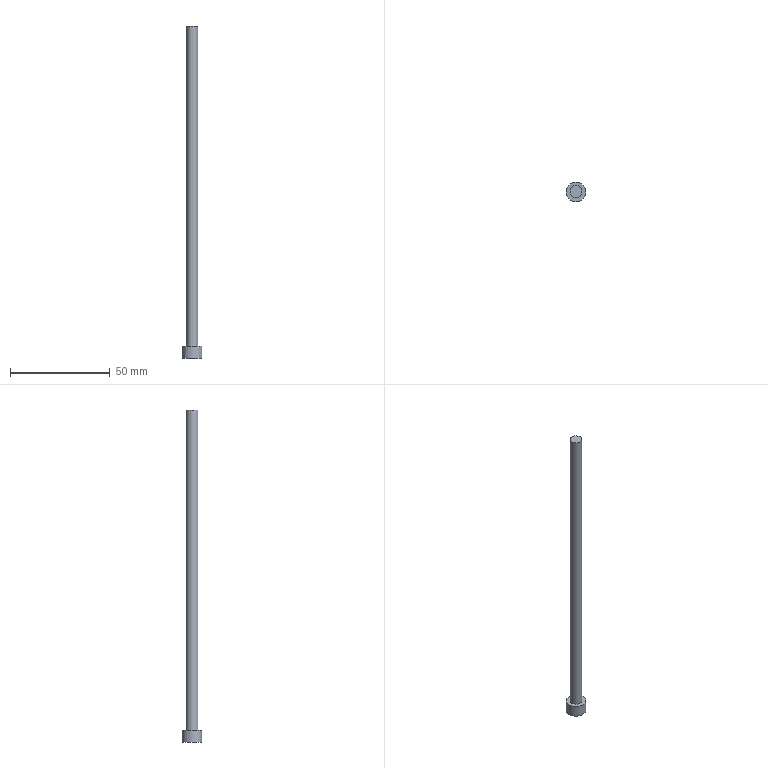Part | STEP file | DDZ6.00_id250_x_t | 1 solid | 5 faces | box 10 x 10 x 166.5 mm | volume 5009 mm3 | plane 3 | cylinder 2 | commonest cylinder face diameters 6 x1 10 x1
STEP:
#1=CARTESIAN_POINT('',(-3.,0.,31.));
#2=VERTEX_POINT('',#1);
#3=CARTESIAN_POINT('',(0.,0.,31.));
#4=DIRECTION('',(0.,0.,-1.));
#5=DIRECTION('',(-1.,0.,0.));
#6=AXIS2_PLACEMENT_3D('',#3,#4,#5);
#7=CIRCLE('',#6,3.);
#8=EDGE_CURVE('',#2,#2,#7,.T.);
#9=ORIENTED_EDGE('',*,*,#8,.F.);
#10=EDGE_LOOP('',(#9));
#11=FACE_OUTER_BOUND('',#10,.T.);
#12=CARTESIAN_POINT('',(0.,0.,31.));
#13=DIRECTION('',(0.,0.,1.));
#14=DIRECTION('',(1.,0.,0.));
#15=AXIS2_PLACEMENT_3D('',#12,#13,#14);
#16=PLANE('',#15);
#17=ADVANCED_FACE('',(#11),#16,.T.);
#18=CARTESIAN_POINT('',(3.,0.,-129.5));
#19=VERTEX_POINT('',#18);
#20=CARTESIAN_POINT('',(0.,0.,-129.5));
#21=DIRECTION('',(0.,0.,-1.));
#22=DIRECTION('',(1.,0.,0.));
#23=AXIS2_PLACEMENT_3D('',#20,#21,#22);
#24=CIRCLE('',#23,3.);
#25=EDGE_CURVE('',#19,#19,#24,.T.);
#26=ORIENTED_EDGE('',*,*,#25,.F.);
#27=EDGE_LOOP('',(#26));
#28=FACE_BOUND('',#27,.T.);
#29=ORIENTED_EDGE('',*,*,#8,.T.);
#30=EDGE_LOOP('',(#29));
#31=FACE_BOUND('',#30,.T.);
#32=CARTESIAN_POINT('',(0.,0.,-140.5));
#33=DIRECTION('',(0.,0.,1.));
#34=DIRECTION('',(1.,0.,0.));
#35=AXIS2_PLACEMENT_3D('',#32,#33,#34);
#36=CYLINDRICAL_SURFACE('',#35,3.);
#37=ADVANCED_FACE('',(#28,#31),#36,.T.);
#38=ORIENTED_EDGE('',*,*,#25,.T.);
#39=EDGE_LOOP('',(#38));
#40=FACE_BOUND('',#39,.T.);
#41=CARTESIAN_POINT('',(-5.,0.,-129.5));
#42=VERTEX_POINT('',#41);
#43=CARTESIAN_POINT('',(0.,0.,-129.5));
#44=DIRECTION('',(0.,0.,-1.));
#45=DIRECTION('',(-1.,0.,0.));
#46=AXIS2_PLACEMENT_3D('',#43,#44,#45);
#47=CIRCLE('',#46,5.);
#48=EDGE_CURVE('',#42,#42,#47,.T.);
#49=ORIENTED_EDGE('',*,*,#48,.F.);
#50=EDGE_LOOP('',(#49));
#51=FACE_BOUND('',#50,.T.);
#52=CARTESIAN_POINT('',(0.,0.,-129.5));
#53=DIRECTION('',(0.,0.,1.));
#54=DIRECTION('',(1.,0.,0.));
#55=AXIS2_PLACEMENT_3D('',#52,#53,#54);
#56=PLANE('',#55);
#57=ADVANCED_FACE('',(#40,#51),#56,.T.);
#58=ORIENTED_EDGE('',*,*,#48,.T.);
#59=EDGE_LOOP('',(#58));
#60=FACE_BOUND('',#59,.T.);
#61=CARTESIAN_POINT('',(5.,0.,-135.5));
#62=VERTEX_POINT('',#61);
#63=CARTESIAN_POINT('',(0.,0.,-135.5));
#64=DIRECTION('',(0.,0.,1.));
#65=DIRECTION('',(1.,0.,0.));
#66=AXIS2_PLACEMENT_3D('',#63,#64,#65);
#67=CIRCLE('',#66,5.);
#68=EDGE_CURVE('',#62,#62,#67,.T.);
#69=ORIENTED_EDGE('',*,*,#68,.T.);
#70=EDGE_LOOP('',(#69));
#71=FACE_BOUND('',#70,.T.);
#72=CARTESIAN_POINT('',(0.,0.,-135.5));
#73=DIRECTION('',(0.,0.,1.));
#74=DIRECTION('',(1.,0.,0.));
#75=AXIS2_PLACEMENT_3D('',#72,#73,#74);
#76=CYLINDRICAL_SURFACE('',#75,5.);
#77=ADVANCED_FACE('',(#60,#71),#76,.T.);
#78=ORIENTED_EDGE('',*,*,#68,.F.);
#79=EDGE_LOOP('',(#78));
#80=FACE_OUTER_BOUND('',#79,.T.);
#81=CARTESIAN_POINT('',(0.,0.,-135.5));
#82=DIRECTION('',(0.,0.,-1.));
#83=DIRECTION('',(-1.,0.,0.));
#84=AXIS2_PLACEMENT_3D('',#81,#82,#83);
#85=PLANE('',#84);
#86=ADVANCED_FACE('',(#80),#85,.T.);
#87=CLOSED_SHELL('',(#17,#37,#57,#77,#86));
#88=MANIFOLD_SOLID_BREP('',#87);
#89=(LENGTH_UNIT()NAMED_UNIT(*)SI_UNIT(.MILLI.,.METRE.));
#90=UNCERTAINTY_MEASURE_WITH_UNIT(LENGTH_MEASURE(0.00002),#89,'','');
#91=(NAMED_UNIT(*)PLANE_ANGLE_UNIT()SI_UNIT($,.RADIAN.));
#92=PLANE_ANGLE_MEASURE_WITH_UNIT(PLANE_ANGLE_MEASURE(0.01745),#91);
#93=DIMENSIONAL_EXPONENTS(0.,0.,0.,0.,0.,0.,0.);
#94=(CONVERSION_BASED_UNIT('DEGREE',#92)NAMED_UNIT(#93)PLANE_ANGLE_UNIT());
#95=(NAMED_UNIT(*)SI_UNIT($,.STERADIAN.)SOLID_ANGLE_UNIT());
#96=(GEOMETRIC_REPRESENTATION_CONTEXT(3)GLOBAL_UNCERTAINTY_ASSIGNED_CONTEXT((#90))GLOBAL_UNIT_ASSIGNED_CONTEXT((#89,#94,#95))REPRESENTATION_CONTEXT('',''));
#97=ADVANCED_BREP_SHAPE_REPRESENTATION('',(#88),#96);